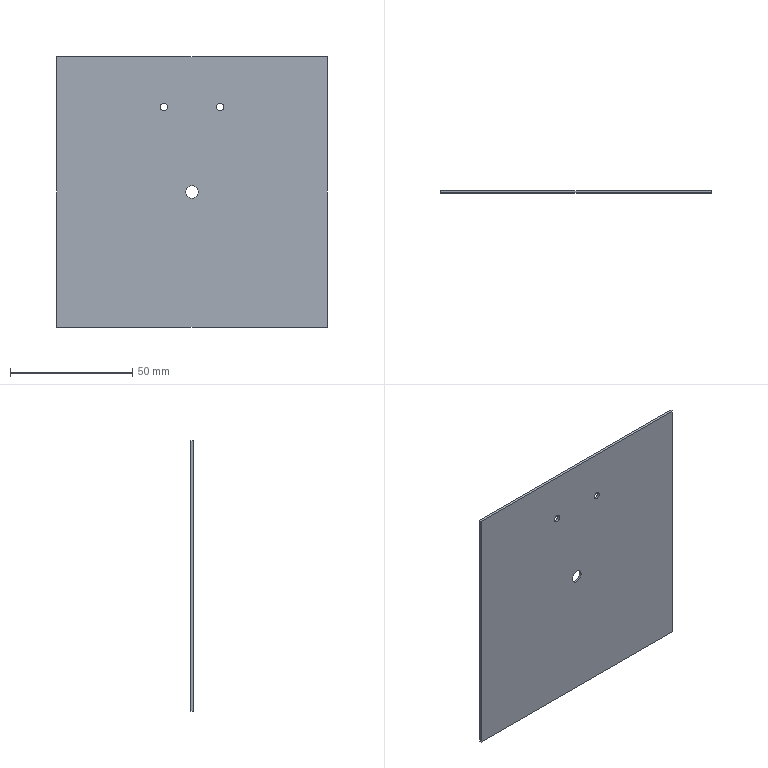Part | SolidWorks | features Extrusion 1 | 1 solid | 12 faces | box 110.5 x 1 x 110.5 mm | volume 12176 mm3 | cylinder 6 | plane 6 | commonest cylinder face diameters 3 x4 5.1 x2
STEP:
#1=CARTESIAN_POINT('',(11.5,1.,33.25));
#2=VERTEX_POINT('',#1);
#3=CARTESIAN_POINT('',(11.5,1.,36.25));
#4=VERTEX_POINT('',#3);
#5=CARTESIAN_POINT('',(11.5,1.,34.75));
#6=DIRECTION('',(0.,1.,0.));
#7=DIRECTION('',(0.,0.,1.));
#8=AXIS2_PLACEMENT_3D('',#5,#6,#7);
#9=CIRCLE('',#8,1.5);
#10=EDGE_CURVE('',#2,#4,#9,.T.);
#11=ORIENTED_EDGE('',*,*,#10,.T.);
#12=CARTESIAN_POINT('',(11.5,0.,36.25));
#13=VERTEX_POINT('',#12);
#14=CARTESIAN_POINT('',(11.5,1.,36.25));
#15=DIRECTION('',(0.,-1.,0.));
#16=VECTOR('',#15,1000.);
#17=LINE('',#14,#16);
#18=EDGE_CURVE('',#4,#13,#17,.T.);
#19=ORIENTED_EDGE('',*,*,#18,.T.);
#20=CARTESIAN_POINT('',(11.5,0.,33.25));
#21=VERTEX_POINT('',#20);
#22=CARTESIAN_POINT('',(11.5,0.,34.75));
#23=DIRECTION('',(0.,1.,0.));
#24=DIRECTION('',(0.,0.,1.));
#25=AXIS2_PLACEMENT_3D('',#22,#23,#24);
#26=CIRCLE('',#25,1.5);
#27=EDGE_CURVE('',#21,#13,#26,.T.);
#28=ORIENTED_EDGE('',*,*,#27,.F.);
#29=CARTESIAN_POINT('',(11.5,1.,33.25));
#30=DIRECTION('',(0.,-1.,0.));
#31=VECTOR('',#30,1000.);
#32=LINE('',#29,#31);
#33=EDGE_CURVE('',#2,#21,#32,.T.);
#34=ORIENTED_EDGE('',*,*,#33,.F.);
#35=EDGE_LOOP('',(#11,#19,#28,#34));
#36=FACE_OUTER_BOUND('',#35,.T.);
#37=CARTESIAN_POINT('',(11.5,1.,34.75));
#38=DIRECTION('',(0.,-1.,0.));
#39=DIRECTION('',(0.,0.,-1.));
#40=AXIS2_PLACEMENT_3D('',#37,#38,#39);
#41=CYLINDRICAL_SURFACE('',#40,1.5);
#42=ADVANCED_FACE('',(#36),#41,.F.);
#43=CARTESIAN_POINT('',(-11.5,1.,33.25));
#44=VERTEX_POINT('',#43);
#45=CARTESIAN_POINT('',(-11.5,1.,36.25));
#46=VERTEX_POINT('',#45);
#47=CARTESIAN_POINT('',(-11.5,1.,34.75));
#48=DIRECTION('',(0.,1.,0.));
#49=DIRECTION('',(0.,0.,1.));
#50=AXIS2_PLACEMENT_3D('',#47,#48,#49);
#51=CIRCLE('',#50,1.5);
#52=EDGE_CURVE('',#44,#46,#51,.T.);
#53=ORIENTED_EDGE('',*,*,#52,.T.);
#54=CARTESIAN_POINT('',(-11.5,0.,36.25));
#55=VERTEX_POINT('',#54);
#56=CARTESIAN_POINT('',(-11.5,1.,36.25));
#57=DIRECTION('',(0.,-1.,0.));
#58=VECTOR('',#57,1000.);
#59=LINE('',#56,#58);
#60=EDGE_CURVE('',#46,#55,#59,.T.);
#61=ORIENTED_EDGE('',*,*,#60,.T.);
#62=CARTESIAN_POINT('',(-11.5,0.,33.25));
#63=VERTEX_POINT('',#62);
#64=CARTESIAN_POINT('',(-11.5,0.,34.75));
#65=DIRECTION('',(0.,1.,0.));
#66=DIRECTION('',(0.,0.,1.));
#67=AXIS2_PLACEMENT_3D('',#64,#65,#66);
#68=CIRCLE('',#67,1.5);
#69=EDGE_CURVE('',#63,#55,#68,.T.);
#70=ORIENTED_EDGE('',*,*,#69,.F.);
#71=CARTESIAN_POINT('',(-11.5,1.,33.25));
#72=DIRECTION('',(0.,-1.,0.));
#73=VECTOR('',#72,1000.);
#74=LINE('',#71,#73);
#75=EDGE_CURVE('',#44,#63,#74,.T.);
#76=ORIENTED_EDGE('',*,*,#75,.F.);
#77=EDGE_LOOP('',(#53,#61,#70,#76));
#78=FACE_OUTER_BOUND('',#77,.T.);
#79=CARTESIAN_POINT('',(-11.5,1.,34.75));
#80=DIRECTION('',(0.,-1.,0.));
#81=DIRECTION('',(0.,0.,-1.));
#82=AXIS2_PLACEMENT_3D('',#79,#80,#81);
#83=CYLINDRICAL_SURFACE('',#82,1.5);
#84=ADVANCED_FACE('',(#78),#83,.F.);
#85=CARTESIAN_POINT('',(0.,1.,-2.55));
#86=VERTEX_POINT('',#85);
#87=CARTESIAN_POINT('',(0.,1.,2.55));
#88=VERTEX_POINT('',#87);
#89=CARTESIAN_POINT('',(0.,1.,0.));
#90=DIRECTION('',(0.,1.,0.));
#91=DIRECTION('',(0.,0.,1.));
#92=AXIS2_PLACEMENT_3D('',#89,#90,#91);
#93=CIRCLE('',#92,2.55);
#94=EDGE_CURVE('',#86,#88,#93,.T.);
#95=ORIENTED_EDGE('',*,*,#94,.T.);
#96=CARTESIAN_POINT('',(0.,0.,2.55));
#97=VERTEX_POINT('',#96);
#98=CARTESIAN_POINT('',(0.,1.,2.55));
#99=DIRECTION('',(0.,-1.,0.));
#100=VECTOR('',#99,1000.);
#101=LINE('',#98,#100);
#102=EDGE_CURVE('',#88,#97,#101,.T.);
#103=ORIENTED_EDGE('',*,*,#102,.T.);
#104=CARTESIAN_POINT('',(0.,0.,-2.55));
#105=VERTEX_POINT('',#104);
#106=CARTESIAN_POINT('',(0.,0.,0.));
#107=DIRECTION('',(0.,1.,0.));
#108=DIRECTION('',(0.,0.,1.));
#109=AXIS2_PLACEMENT_3D('',#106,#107,#108);
#110=CIRCLE('',#109,2.55);
#111=EDGE_CURVE('',#105,#97,#110,.T.);
#112=ORIENTED_EDGE('',*,*,#111,.F.);
#113=CARTESIAN_POINT('',(0.,1.,-2.55));
#114=DIRECTION('',(0.,-1.,0.));
#115=VECTOR('',#114,1000.);
#116=LINE('',#113,#115);
#117=EDGE_CURVE('',#86,#105,#116,.T.);
#118=ORIENTED_EDGE('',*,*,#117,.F.);
#119=EDGE_LOOP('',(#95,#103,#112,#118));
#120=FACE_OUTER_BOUND('',#119,.T.);
#121=CARTESIAN_POINT('',(0.,1.,0.));
#122=DIRECTION('',(0.,-1.,0.));
#123=DIRECTION('',(0.,0.,-1.));
#124=AXIS2_PLACEMENT_3D('',#121,#122,#123);
#125=CYLINDRICAL_SURFACE('',#124,2.55);
#126=ADVANCED_FACE('',(#120),#125,.F.);
#127=ORIENTED_EDGE('',*,*,#52,.F.);
#128=CARTESIAN_POINT('',(-11.5,1.,34.75));
#129=DIRECTION('',(0.,1.,0.));
#130=DIRECTION('',(0.,0.,1.));
#131=AXIS2_PLACEMENT_3D('',#128,#129,#130);
#132=CIRCLE('',#131,1.5);
#133=EDGE_CURVE('',#46,#44,#132,.T.);
#134=ORIENTED_EDGE('',*,*,#133,.F.);
#135=EDGE_LOOP('',(#127,#134));
#136=FACE_BOUND('',#135,.T.);
#137=CARTESIAN_POINT('',(55.25,1.,55.25));
#138=VERTEX_POINT('',#137);
#139=CARTESIAN_POINT('',(55.25,1.,-55.25));
#140=VERTEX_POINT('',#139);
#141=CARTESIAN_POINT('',(55.25,1.,55.25));
#142=DIRECTION('',(0.,0.,-1.));
#143=VECTOR('',#142,1000.);
#144=LINE('',#141,#143);
#145=EDGE_CURVE('',#138,#140,#144,.T.);
#146=ORIENTED_EDGE('',*,*,#145,.T.);
#147=CARTESIAN_POINT('',(-55.25,1.,-55.25));
#148=VERTEX_POINT('',#147);
#149=CARTESIAN_POINT('',(-55.25,1.,-55.25));
#150=DIRECTION('',(-1.,0.,0.));
#151=VECTOR('',#150,1000.);
#152=LINE('',#149,#151);
#153=EDGE_CURVE('',#140,#148,#152,.T.);
#154=ORIENTED_EDGE('',*,*,#153,.T.);
#155=CARTESIAN_POINT('',(-55.25,1.,55.25));
#156=VERTEX_POINT('',#155);
#157=CARTESIAN_POINT('',(-55.25,1.,55.25));
#158=DIRECTION('',(0.,0.,1.));
#159=VECTOR('',#158,1000.);
#160=LINE('',#157,#159);
#161=EDGE_CURVE('',#148,#156,#160,.T.);
#162=ORIENTED_EDGE('',*,*,#161,.T.);
#163=CARTESIAN_POINT('',(-55.25,1.,55.25));
#164=DIRECTION('',(1.,0.,0.));
#165=VECTOR('',#164,1000.);
#166=LINE('',#163,#165);
#167=EDGE_CURVE('',#156,#138,#166,.T.);
#168=ORIENTED_EDGE('',*,*,#167,.T.);
#169=EDGE_LOOP('',(#146,#154,#162,#168));
#170=FACE_OUTER_BOUND('',#169,.T.);
#171=ORIENTED_EDGE('',*,*,#94,.F.);
#172=CARTESIAN_POINT('',(0.,1.,0.));
#173=DIRECTION('',(0.,1.,0.));
#174=DIRECTION('',(0.,0.,1.));
#175=AXIS2_PLACEMENT_3D('',#172,#173,#174);
#176=CIRCLE('',#175,2.55);
#177=EDGE_CURVE('',#88,#86,#176,.T.);
#178=ORIENTED_EDGE('',*,*,#177,.F.);
#179=EDGE_LOOP('',(#171,#178));
#180=FACE_BOUND('',#179,.T.);
#181=ORIENTED_EDGE('',*,*,#10,.F.);
#182=CARTESIAN_POINT('',(11.5,1.,34.75));
#183=DIRECTION('',(0.,1.,0.));
#184=DIRECTION('',(0.,0.,1.));
#185=AXIS2_PLACEMENT_3D('',#182,#183,#184);
#186=CIRCLE('',#185,1.5);
#187=EDGE_CURVE('',#4,#2,#186,.T.);
#188=ORIENTED_EDGE('',*,*,#187,.F.);
#189=EDGE_LOOP('',(#181,#188));
#190=FACE_BOUND('',#189,.T.);
#191=CARTESIAN_POINT('',(0.,1.,0.));
#192=DIRECTION('',(0.,-1.,0.));
#193=DIRECTION('',(0.,0.,-1.));
#194=AXIS2_PLACEMENT_3D('',#191,#192,#193);
#195=PLANE('',#194);
#196=ADVANCED_FACE('',(#136,#170,#180,#190),#195,.F.);
#197=ORIENTED_EDGE('',*,*,#69,.T.);
#198=CARTESIAN_POINT('',(-11.5,0.,34.75));
#199=DIRECTION('',(0.,1.,0.));
#200=DIRECTION('',(0.,0.,1.));
#201=AXIS2_PLACEMENT_3D('',#198,#199,#200);
#202=CIRCLE('',#201,1.5);
#203=EDGE_CURVE('',#55,#63,#202,.T.);
#204=ORIENTED_EDGE('',*,*,#203,.T.);
#205=EDGE_LOOP('',(#197,#204));
#206=FACE_BOUND('',#205,.T.);
#207=CARTESIAN_POINT('',(55.25,0.,55.25));
#208=VERTEX_POINT('',#207);
#209=CARTESIAN_POINT('',(55.25,0.,-55.25));
#210=VERTEX_POINT('',#209);
#211=CARTESIAN_POINT('',(55.25,0.,55.25));
#212=DIRECTION('',(0.,0.,-1.));
#213=VECTOR('',#212,1000.);
#214=LINE('',#211,#213);
#215=EDGE_CURVE('',#208,#210,#214,.T.);
#216=ORIENTED_EDGE('',*,*,#215,.F.);
#217=CARTESIAN_POINT('',(-55.25,0.,55.25));
#218=VERTEX_POINT('',#217);
#219=CARTESIAN_POINT('',(-55.25,0.,55.25));
#220=DIRECTION('',(1.,0.,0.));
#221=VECTOR('',#220,1000.);
#222=LINE('',#219,#221);
#223=EDGE_CURVE('',#218,#208,#222,.T.);
#224=ORIENTED_EDGE('',*,*,#223,.F.);
#225=CARTESIAN_POINT('',(-55.25,0.,-55.25));
#226=VERTEX_POINT('',#225);
#227=CARTESIAN_POINT('',(-55.25,0.,55.25));
#228=DIRECTION('',(0.,0.,1.));
#229=VECTOR('',#228,1000.);
#230=LINE('',#227,#229);
#231=EDGE_CURVE('',#226,#218,#230,.T.);
#232=ORIENTED_EDGE('',*,*,#231,.F.);
#233=CARTESIAN_POINT('',(-55.25,0.,-55.25));
#234=DIRECTION('',(-1.,0.,0.));
#235=VECTOR('',#234,1000.);
#236=LINE('',#233,#235);
#237=EDGE_CURVE('',#210,#226,#236,.T.);
#238=ORIENTED_EDGE('',*,*,#237,.F.);
#239=EDGE_LOOP('',(#216,#224,#232,#238));
#240=FACE_OUTER_BOUND('',#239,.T.);
#241=ORIENTED_EDGE('',*,*,#111,.T.);
#242=CARTESIAN_POINT('',(0.,0.,0.));
#243=DIRECTION('',(0.,1.,0.));
#244=DIRECTION('',(0.,0.,1.));
#245=AXIS2_PLACEMENT_3D('',#242,#243,#244);
#246=CIRCLE('',#245,2.55);
#247=EDGE_CURVE('',#97,#105,#246,.T.);
#248=ORIENTED_EDGE('',*,*,#247,.T.);
#249=EDGE_LOOP('',(#241,#248));
#250=FACE_BOUND('',#249,.T.);
#251=ORIENTED_EDGE('',*,*,#27,.T.);
#252=CARTESIAN_POINT('',(11.5,0.,34.75));
#253=DIRECTION('',(0.,1.,0.));
#254=DIRECTION('',(0.,0.,1.));
#255=AXIS2_PLACEMENT_3D('',#252,#253,#254);
#256=CIRCLE('',#255,1.5);
#257=EDGE_CURVE('',#13,#21,#256,.T.);
#258=ORIENTED_EDGE('',*,*,#257,.T.);
#259=EDGE_LOOP('',(#251,#258));
#260=FACE_BOUND('',#259,.T.);
#261=CARTESIAN_POINT('',(0.,0.,0.));
#262=DIRECTION('',(0.,-1.,0.));
#263=DIRECTION('',(0.,0.,-1.));
#264=AXIS2_PLACEMENT_3D('',#261,#262,#263);
#265=PLANE('',#264);
#266=ADVANCED_FACE('',(#206,#240,#250,#260),#265,.T.);
#267=ORIENTED_EDGE('',*,*,#215,.T.);
#268=CARTESIAN_POINT('',(55.25,1.,-55.25));
#269=DIRECTION('',(0.,-1.,0.));
#270=VECTOR('',#269,1000.);
#271=LINE('',#268,#270);
#272=EDGE_CURVE('',#140,#210,#271,.T.);
#273=ORIENTED_EDGE('',*,*,#272,.F.);
#274=ORIENTED_EDGE('',*,*,#145,.F.);
#275=CARTESIAN_POINT('',(55.25,1.,55.25));
#276=DIRECTION('',(0.,-1.,0.));
#277=VECTOR('',#276,1000.);
#278=LINE('',#275,#277);
#279=EDGE_CURVE('',#138,#208,#278,.T.);
#280=ORIENTED_EDGE('',*,*,#279,.T.);
#281=EDGE_LOOP('',(#267,#273,#274,#280));
#282=FACE_OUTER_BOUND('',#281,.T.);
#283=CARTESIAN_POINT('',(55.25,1.,55.25));
#284=DIRECTION('',(-1.,0.,0.));
#285=DIRECTION('',(0.,0.,1.));
#286=AXIS2_PLACEMENT_3D('',#283,#284,#285);
#287=PLANE('',#286);
#288=ADVANCED_FACE('',(#282),#287,.F.);
#289=ORIENTED_EDGE('',*,*,#237,.T.);
#290=CARTESIAN_POINT('',(-55.25,1.,-55.25));
#291=DIRECTION('',(0.,-1.,0.));
#292=VECTOR('',#291,1000.);
#293=LINE('',#290,#292);
#294=EDGE_CURVE('',#148,#226,#293,.T.);
#295=ORIENTED_EDGE('',*,*,#294,.F.);
#296=ORIENTED_EDGE('',*,*,#153,.F.);
#297=ORIENTED_EDGE('',*,*,#272,.T.);
#298=EDGE_LOOP('',(#289,#295,#296,#297));
#299=FACE_OUTER_BOUND('',#298,.T.);
#300=CARTESIAN_POINT('',(-55.25,1.,-55.25));
#301=DIRECTION('',(0.,0.,1.));
#302=DIRECTION('',(1.,0.,0.));
#303=AXIS2_PLACEMENT_3D('',#300,#301,#302);
#304=PLANE('',#303);
#305=ADVANCED_FACE('',(#299),#304,.F.);
#306=ORIENTED_EDGE('',*,*,#231,.T.);
#307=CARTESIAN_POINT('',(-55.25,1.,55.25));
#308=DIRECTION('',(0.,-1.,0.));
#309=VECTOR('',#308,1000.);
#310=LINE('',#307,#309);
#311=EDGE_CURVE('',#156,#218,#310,.T.);
#312=ORIENTED_EDGE('',*,*,#311,.F.);
#313=ORIENTED_EDGE('',*,*,#161,.F.);
#314=ORIENTED_EDGE('',*,*,#294,.T.);
#315=EDGE_LOOP('',(#306,#312,#313,#314));
#316=FACE_OUTER_BOUND('',#315,.T.);
#317=CARTESIAN_POINT('',(-55.25,1.,55.25));
#318=DIRECTION('',(1.,0.,0.));
#319=DIRECTION('',(0.,0.,-1.));
#320=AXIS2_PLACEMENT_3D('',#317,#318,#319);
#321=PLANE('',#320);
#322=ADVANCED_FACE('',(#316),#321,.F.);
#323=ORIENTED_EDGE('',*,*,#223,.T.);
#324=ORIENTED_EDGE('',*,*,#279,.F.);
#325=ORIENTED_EDGE('',*,*,#167,.F.);
#326=ORIENTED_EDGE('',*,*,#311,.T.);
#327=EDGE_LOOP('',(#323,#324,#325,#326));
#328=FACE_OUTER_BOUND('',#327,.T.);
#329=CARTESIAN_POINT('',(-55.25,1.,55.25));
#330=DIRECTION('',(0.,0.,-1.));
#331=DIRECTION('',(-1.,0.,0.));
#332=AXIS2_PLACEMENT_3D('',#329,#330,#331);
#333=PLANE('',#332);
#334=ADVANCED_FACE('',(#328),#333,.F.);
#335=ORIENTED_EDGE('',*,*,#102,.F.);
#336=ORIENTED_EDGE('',*,*,#177,.T.);
#337=ORIENTED_EDGE('',*,*,#117,.T.);
#338=ORIENTED_EDGE('',*,*,#247,.F.);
#339=EDGE_LOOP('',(#335,#336,#337,#338));
#340=FACE_OUTER_BOUND('',#339,.T.);
#341=CARTESIAN_POINT('',(0.,1.,0.));
#342=DIRECTION('',(0.,-1.,0.));
#343=DIRECTION('',(0.,0.,-1.));
#344=AXIS2_PLACEMENT_3D('',#341,#342,#343);
#345=CYLINDRICAL_SURFACE('',#344,2.55);
#346=ADVANCED_FACE('',(#340),#345,.F.);
#347=ORIENTED_EDGE('',*,*,#60,.F.);
#348=ORIENTED_EDGE('',*,*,#133,.T.);
#349=ORIENTED_EDGE('',*,*,#75,.T.);
#350=ORIENTED_EDGE('',*,*,#203,.F.);
#351=EDGE_LOOP('',(#347,#348,#349,#350));
#352=FACE_OUTER_BOUND('',#351,.T.);
#353=CARTESIAN_POINT('',(-11.5,1.,34.75));
#354=DIRECTION('',(0.,-1.,0.));
#355=DIRECTION('',(0.,0.,-1.));
#356=AXIS2_PLACEMENT_3D('',#353,#354,#355);
#357=CYLINDRICAL_SURFACE('',#356,1.5);
#358=ADVANCED_FACE('',(#352),#357,.F.);
#359=ORIENTED_EDGE('',*,*,#18,.F.);
#360=ORIENTED_EDGE('',*,*,#187,.T.);
#361=ORIENTED_EDGE('',*,*,#33,.T.);
#362=ORIENTED_EDGE('',*,*,#257,.F.);
#363=EDGE_LOOP('',(#359,#360,#361,#362));
#364=FACE_OUTER_BOUND('',#363,.T.);
#365=CARTESIAN_POINT('',(11.5,1.,34.75));
#366=DIRECTION('',(0.,-1.,0.));
#367=DIRECTION('',(0.,0.,-1.));
#368=AXIS2_PLACEMENT_3D('',#365,#366,#367);
#369=CYLINDRICAL_SURFACE('',#368,1.5);
#370=ADVANCED_FACE('',(#364),#369,.F.);
#371=CLOSED_SHELL('',(#42,#84,#126,#196,#266,#288,#305,#322,#334,#346,#358,#370));
#372=MANIFOLD_SOLID_BREP('',#371);
#373=CARTESIAN_POINT('',(0.,0.,0.));
#374=DIRECTION('',(0.,0.,1.));
#375=DIRECTION('',(1.,0.,0.));
#376=AXIS2_PLACEMENT_3D('',#373,#374,#375);
#377=(LENGTH_UNIT()NAMED_UNIT(*)SI_UNIT(.MILLI.,.METRE.));
#378=UNCERTAINTY_MEASURE_WITH_UNIT(LENGTH_MEASURE(0.00001),#377,'','');
#379=(NAMED_UNIT(*)PLANE_ANGLE_UNIT()SI_UNIT($,.RADIAN.));
#380=(NAMED_UNIT(*)SI_UNIT($,.STERADIAN.)SOLID_ANGLE_UNIT());
#381=(GEOMETRIC_REPRESENTATION_CONTEXT(3)GLOBAL_UNCERTAINTY_ASSIGNED_CONTEXT((#378))GLOBAL_UNIT_ASSIGNED_CONTEXT((#377,#379,#380))REPRESENTATION_CONTEXT('',''));
#382=ADVANCED_BREP_SHAPE_REPRESENTATION('',(#372,#376),#381);